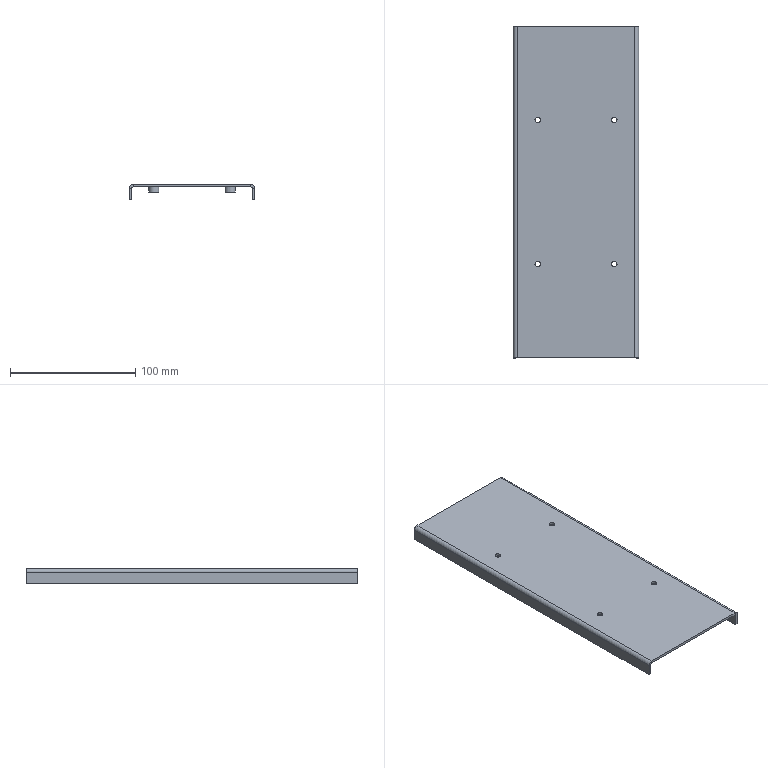Part | SolidWorks | features BaseBody 1 | 1 solid | 54 faces | box 100 x 265 x 12 mm | volume 63166 mm3 | cylinder 28 | plane 26 | commonest cylinder face diameters 4 x8 4.5 x8 8 x8 2 x2 6 x2
STEP:
#1=CARTESIAN_POINT('',(-32.5,-57.5,-6.));
#2=VERTEX_POINT('',#1);
#3=CARTESIAN_POINT('',(-32.5,-57.5,-2.));
#4=VERTEX_POINT('',#3);
#5=CARTESIAN_POINT('',(-32.5,-57.5,-6.));
#6=DIRECTION('',(0.,0.,1.));
#7=VECTOR('',#6,1000.);
#8=LINE('',#5,#7);
#9=EDGE_CURVE('',#2,#4,#8,.T.);
#10=ORIENTED_EDGE('',*,*,#9,.F.);
#11=CARTESIAN_POINT('',(-28.5,-57.5,-6.));
#12=VERTEX_POINT('',#11);
#13=CARTESIAN_POINT('',(-30.5,-57.5,-6.));
#14=DIRECTION('',(0.,0.,-1.));
#15=DIRECTION('',(-1.,0.,0.));
#16=AXIS2_PLACEMENT_3D('',#13,#14,#15);
#17=CIRCLE('',#16,2.);
#18=EDGE_CURVE('',#2,#12,#17,.T.);
#19=ORIENTED_EDGE('',*,*,#18,.T.);
#20=CARTESIAN_POINT('',(-28.5,-57.5,-2.));
#21=VERTEX_POINT('',#20);
#22=CARTESIAN_POINT('',(-28.5,-57.5,-6.));
#23=DIRECTION('',(0.,0.,1.));
#24=VECTOR('',#23,1000.);
#25=LINE('',#22,#24);
#26=EDGE_CURVE('',#12,#21,#25,.T.);
#27=ORIENTED_EDGE('',*,*,#26,.T.);
#28=CARTESIAN_POINT('',(-30.5,-57.5,-2.));
#29=DIRECTION('',(0.,0.,-1.));
#30=DIRECTION('',(-1.,0.,0.));
#31=AXIS2_PLACEMENT_3D('',#28,#29,#30);
#32=CIRCLE('',#31,2.);
#33=EDGE_CURVE('',#4,#21,#32,.T.);
#34=ORIENTED_EDGE('',*,*,#33,.F.);
#35=EDGE_LOOP('',(#10,#19,#27,#34));
#36=FACE_OUTER_BOUND('',#35,.T.);
#37=CARTESIAN_POINT('',(-30.5,-57.5,-6.));
#38=DIRECTION('',(0.,0.,1.));
#39=DIRECTION('',(1.,0.,0.));
#40=AXIS2_PLACEMENT_3D('',#37,#38,#39);
#41=CYLINDRICAL_SURFACE('',#40,2.);
#42=ADVANCED_FACE('',(#36),#41,.F.);
#43=CARTESIAN_POINT('',(-34.5,-57.5,-6.));
#44=VERTEX_POINT('',#43);
#45=CARTESIAN_POINT('',(-34.5,-57.5,-2.));
#46=VERTEX_POINT('',#45);
#47=CARTESIAN_POINT('',(-34.5,-57.5,-6.));
#48=DIRECTION('',(0.,0.,1.));
#49=VECTOR('',#48,1000.);
#50=LINE('',#47,#49);
#51=EDGE_CURVE('',#44,#46,#50,.T.);
#52=ORIENTED_EDGE('',*,*,#51,.F.);
#53=CARTESIAN_POINT('',(-26.5,-57.5,-6.));
#54=VERTEX_POINT('',#53);
#55=CARTESIAN_POINT('',(-30.5,-57.5,-6.));
#56=DIRECTION('',(0.,0.,-1.));
#57=DIRECTION('',(-1.,0.,0.));
#58=AXIS2_PLACEMENT_3D('',#55,#56,#57);
#59=CIRCLE('',#58,4.);
#60=EDGE_CURVE('',#54,#44,#59,.T.);
#61=ORIENTED_EDGE('',*,*,#60,.F.);
#62=CARTESIAN_POINT('',(-26.5,-57.5,-2.));
#63=VERTEX_POINT('',#62);
#64=CARTESIAN_POINT('',(-26.5,-57.5,-6.));
#65=DIRECTION('',(0.,0.,1.));
#66=VECTOR('',#65,1000.);
#67=LINE('',#64,#66);
#68=EDGE_CURVE('',#54,#63,#67,.T.);
#69=ORIENTED_EDGE('',*,*,#68,.T.);
#70=CARTESIAN_POINT('',(-30.5,-57.5,-2.));
#71=DIRECTION('',(0.,0.,-1.));
#72=DIRECTION('',(1.,0.,0.));
#73=AXIS2_PLACEMENT_3D('',#70,#71,#72);
#74=CIRCLE('',#73,4.);
#75=EDGE_CURVE('',#63,#46,#74,.T.);
#76=ORIENTED_EDGE('',*,*,#75,.T.);
#77=EDGE_LOOP('',(#52,#61,#69,#76));
#78=FACE_OUTER_BOUND('',#77,.T.);
#79=CARTESIAN_POINT('',(-30.5,-57.5,-6.));
#80=DIRECTION('',(0.,0.,1.));
#81=DIRECTION('',(1.,0.,0.));
#82=AXIS2_PLACEMENT_3D('',#79,#80,#81);
#83=CYLINDRICAL_SURFACE('',#82,4.);
#84=ADVANCED_FACE('',(#78),#83,.T.);
#85=CARTESIAN_POINT('',(-30.5,-57.5,-6.));
#86=DIRECTION('',(0.,0.,-1.));
#87=DIRECTION('',(-1.,0.,0.));
#88=AXIS2_PLACEMENT_3D('',#85,#86,#87);
#89=CIRCLE('',#88,2.);
#90=EDGE_CURVE('',#12,#2,#89,.T.);
#91=ORIENTED_EDGE('',*,*,#90,.F.);
#92=ORIENTED_EDGE('',*,*,#18,.F.);
#93=EDGE_LOOP('',(#91,#92));
#94=FACE_BOUND('',#93,.T.);
#95=ORIENTED_EDGE('',*,*,#60,.T.);
#96=CARTESIAN_POINT('',(-30.5,-57.5,-6.));
#97=DIRECTION('',(0.,0.,-1.));
#98=DIRECTION('',(-1.,0.,0.));
#99=AXIS2_PLACEMENT_3D('',#96,#97,#98);
#100=CIRCLE('',#99,4.);
#101=EDGE_CURVE('',#44,#54,#100,.T.);
#102=ORIENTED_EDGE('',*,*,#101,.T.);
#103=EDGE_LOOP('',(#95,#102));
#104=FACE_OUTER_BOUND('',#103,.T.);
#105=CARTESIAN_POINT('',(-30.5,-57.5,-6.));
#106=DIRECTION('',(0.,0.,-1.));
#107=DIRECTION('',(0.,-1.,0.));
#108=AXIS2_PLACEMENT_3D('',#105,#106,#107);
#109=PLANE('',#108);
#110=ADVANCED_FACE('',(#94,#104),#109,.T.);
#111=CARTESIAN_POINT('',(-30.5,-57.5,-2.));
#112=DIRECTION('',(0.,0.,-1.));
#113=DIRECTION('',(-1.,0.,0.));
#114=AXIS2_PLACEMENT_3D('',#111,#112,#113);
#115=CIRCLE('',#114,2.);
#116=EDGE_CURVE('',#21,#4,#115,.T.);
#117=ORIENTED_EDGE('',*,*,#116,.T.);
#118=ORIENTED_EDGE('',*,*,#33,.T.);
#119=EDGE_LOOP('',(#117,#118));
#120=FACE_BOUND('',#119,.T.);
#121=CARTESIAN_POINT('',(-28.25,-57.5,-2.));
#122=VERTEX_POINT('',#121);
#123=CARTESIAN_POINT('',(-32.75,-57.5,-2.));
#124=VERTEX_POINT('',#123);
#125=CARTESIAN_POINT('',(-30.5,-57.5,-2.));
#126=DIRECTION('',(0.,0.,1.));
#127=DIRECTION('',(1.,0.,0.));
#128=AXIS2_PLACEMENT_3D('',#125,#126,#127);
#129=CIRCLE('',#128,2.25);
#130=EDGE_CURVE('',#122,#124,#129,.T.);
#131=ORIENTED_EDGE('',*,*,#130,.T.);
#132=CARTESIAN_POINT('',(-30.5,-57.5,-2.));
#133=DIRECTION('',(0.,0.,1.));
#134=DIRECTION('',(1.,0.,0.));
#135=AXIS2_PLACEMENT_3D('',#132,#133,#134);
#136=CIRCLE('',#135,2.25);
#137=EDGE_CURVE('',#124,#122,#136,.T.);
#138=ORIENTED_EDGE('',*,*,#137,.T.);
#139=EDGE_LOOP('',(#131,#138));
#140=FACE_OUTER_BOUND('',#139,.T.);
#141=CARTESIAN_POINT('',(-30.5,-57.5,-2.));
#142=DIRECTION('',(0.,0.,-1.));
#143=DIRECTION('',(0.,-1.,0.));
#144=AXIS2_PLACEMENT_3D('',#141,#142,#143);
#145=PLANE('',#144);
#146=ADVANCED_FACE('',(#120,#140),#145,.F.);
#147=CARTESIAN_POINT('',(28.5,-57.5,-6.));
#148=VERTEX_POINT('',#147);
#149=CARTESIAN_POINT('',(28.5,-57.5,-2.));
#150=VERTEX_POINT('',#149);
#151=CARTESIAN_POINT('',(28.5,-57.5,-6.));
#152=DIRECTION('',(0.,0.,1.));
#153=VECTOR('',#152,1000.);
#154=LINE('',#151,#153);
#155=EDGE_CURVE('',#148,#150,#154,.T.);
#156=ORIENTED_EDGE('',*,*,#155,.F.);
#157=CARTESIAN_POINT('',(32.5,-57.5,-6.));
#158=VERTEX_POINT('',#157);
#159=CARTESIAN_POINT('',(30.5,-57.5,-6.));
#160=DIRECTION('',(0.,0.,-1.));
#161=DIRECTION('',(-1.,0.,0.));
#162=AXIS2_PLACEMENT_3D('',#159,#160,#161);
#163=CIRCLE('',#162,2.);
#164=EDGE_CURVE('',#148,#158,#163,.T.);
#165=ORIENTED_EDGE('',*,*,#164,.T.);
#166=CARTESIAN_POINT('',(32.5,-57.5,-2.));
#167=VERTEX_POINT('',#166);
#168=CARTESIAN_POINT('',(32.5,-57.5,-6.));
#169=DIRECTION('',(0.,0.,1.));
#170=VECTOR('',#169,1000.);
#171=LINE('',#168,#170);
#172=EDGE_CURVE('',#158,#167,#171,.T.);
#173=ORIENTED_EDGE('',*,*,#172,.T.);
#174=CARTESIAN_POINT('',(30.5,-57.5,-2.));
#175=DIRECTION('',(0.,0.,-1.));
#176=DIRECTION('',(-1.,0.,0.));
#177=AXIS2_PLACEMENT_3D('',#174,#175,#176);
#178=CIRCLE('',#177,2.);
#179=EDGE_CURVE('',#150,#167,#178,.T.);
#180=ORIENTED_EDGE('',*,*,#179,.F.);
#181=EDGE_LOOP('',(#156,#165,#173,#180));
#182=FACE_OUTER_BOUND('',#181,.T.);
#183=CARTESIAN_POINT('',(30.5,-57.5,-6.));
#184=DIRECTION('',(0.,0.,1.));
#185=DIRECTION('',(1.,0.,0.));
#186=AXIS2_PLACEMENT_3D('',#183,#184,#185);
#187=CYLINDRICAL_SURFACE('',#186,2.);
#188=ADVANCED_FACE('',(#182),#187,.F.);
#189=CARTESIAN_POINT('',(26.5,-57.5,-6.));
#190=VERTEX_POINT('',#189);
#191=CARTESIAN_POINT('',(26.5,-57.5,-2.));
#192=VERTEX_POINT('',#191);
#193=CARTESIAN_POINT('',(26.5,-57.5,-6.));
#194=DIRECTION('',(0.,0.,1.));
#195=VECTOR('',#194,1000.);
#196=LINE('',#193,#195);
#197=EDGE_CURVE('',#190,#192,#196,.T.);
#198=ORIENTED_EDGE('',*,*,#197,.F.);
#199=CARTESIAN_POINT('',(34.5,-57.5,-6.));
#200=VERTEX_POINT('',#199);
#201=CARTESIAN_POINT('',(30.5,-57.5,-6.));
#202=DIRECTION('',(0.,0.,-1.));
#203=DIRECTION('',(-1.,0.,0.));
#204=AXIS2_PLACEMENT_3D('',#201,#202,#203);
#205=CIRCLE('',#204,4.);
#206=EDGE_CURVE('',#200,#190,#205,.T.);
#207=ORIENTED_EDGE('',*,*,#206,.F.);
#208=CARTESIAN_POINT('',(34.5,-57.5,-2.));
#209=VERTEX_POINT('',#208);
#210=CARTESIAN_POINT('',(34.5,-57.5,-6.));
#211=DIRECTION('',(0.,0.,1.));
#212=VECTOR('',#211,1000.);
#213=LINE('',#210,#212);
#214=EDGE_CURVE('',#200,#209,#213,.T.);
#215=ORIENTED_EDGE('',*,*,#214,.T.);
#216=CARTESIAN_POINT('',(30.5,-57.5,-2.));
#217=DIRECTION('',(0.,0.,-1.));
#218=DIRECTION('',(1.,0.,0.));
#219=AXIS2_PLACEMENT_3D('',#216,#217,#218);
#220=CIRCLE('',#219,4.);
#221=EDGE_CURVE('',#209,#192,#220,.T.);
#222=ORIENTED_EDGE('',*,*,#221,.T.);
#223=EDGE_LOOP('',(#198,#207,#215,#222));
#224=FACE_OUTER_BOUND('',#223,.T.);
#225=CARTESIAN_POINT('',(30.5,-57.5,-6.));
#226=DIRECTION('',(0.,0.,1.));
#227=DIRECTION('',(1.,0.,0.));
#228=AXIS2_PLACEMENT_3D('',#225,#226,#227);
#229=CYLINDRICAL_SURFACE('',#228,4.);
#230=ADVANCED_FACE('',(#224),#229,.T.);
#231=CARTESIAN_POINT('',(30.5,-57.5,-6.));
#232=DIRECTION('',(0.,0.,-1.));
#233=DIRECTION('',(-1.,0.,0.));
#234=AXIS2_PLACEMENT_3D('',#231,#232,#233);
#235=CIRCLE('',#234,2.);
#236=EDGE_CURVE('',#158,#148,#235,.T.);
#237=ORIENTED_EDGE('',*,*,#236,.F.);
#238=ORIENTED_EDGE('',*,*,#164,.F.);
#239=EDGE_LOOP('',(#237,#238));
#240=FACE_BOUND('',#239,.T.);
#241=ORIENTED_EDGE('',*,*,#206,.T.);
#242=CARTESIAN_POINT('',(30.5,-57.5,-6.));
#243=DIRECTION('',(0.,0.,-1.));
#244=DIRECTION('',(-1.,0.,0.));
#245=AXIS2_PLACEMENT_3D('',#242,#243,#244);
#246=CIRCLE('',#245,4.);
#247=EDGE_CURVE('',#190,#200,#246,.T.);
#248=ORIENTED_EDGE('',*,*,#247,.T.);
#249=EDGE_LOOP('',(#241,#248));
#250=FACE_OUTER_BOUND('',#249,.T.);
#251=CARTESIAN_POINT('',(30.5,-57.5,-6.));
#252=DIRECTION('',(0.,0.,-1.));
#253=DIRECTION('',(0.,-1.,0.));
#254=AXIS2_PLACEMENT_3D('',#251,#252,#253);
#255=PLANE('',#254);
#256=ADVANCED_FACE('',(#240,#250),#255,.T.);
#257=CARTESIAN_POINT('',(30.5,-57.5,-2.));
#258=DIRECTION('',(0.,0.,-1.));
#259=DIRECTION('',(-1.,0.,0.));
#260=AXIS2_PLACEMENT_3D('',#257,#258,#259);
#261=CIRCLE('',#260,2.);
#262=EDGE_CURVE('',#167,#150,#261,.T.);
#263=ORIENTED_EDGE('',*,*,#262,.T.);
#264=ORIENTED_EDGE('',*,*,#179,.T.);
#265=EDGE_LOOP('',(#263,#264));
#266=FACE_BOUND('',#265,.T.);
#267=CARTESIAN_POINT('',(32.75,-57.5,-2.));
#268=VERTEX_POINT('',#267);
#269=CARTESIAN_POINT('',(28.25,-57.5,-2.));
#270=VERTEX_POINT('',#269);
#271=CARTESIAN_POINT('',(30.5,-57.5,-2.));
#272=DIRECTION('',(0.,0.,1.));
#273=DIRECTION('',(1.,0.,0.));
#274=AXIS2_PLACEMENT_3D('',#271,#272,#273);
#275=CIRCLE('',#274,2.25);
#276=EDGE_CURVE('',#268,#270,#275,.T.);
#277=ORIENTED_EDGE('',*,*,#276,.T.);
#278=CARTESIAN_POINT('',(30.5,-57.5,-2.));
#279=DIRECTION('',(0.,0.,1.));
#280=DIRECTION('',(1.,0.,0.));
#281=AXIS2_PLACEMENT_3D('',#278,#279,#280);
#282=CIRCLE('',#281,2.25);
#283=EDGE_CURVE('',#270,#268,#282,.T.);
#284=ORIENTED_EDGE('',*,*,#283,.T.);
#285=EDGE_LOOP('',(#277,#284));
#286=FACE_OUTER_BOUND('',#285,.T.);
#287=CARTESIAN_POINT('',(30.5,-57.5,-2.));
#288=DIRECTION('',(0.,0.,-1.));
#289=DIRECTION('',(0.,-1.,0.));
#290=AXIS2_PLACEMENT_3D('',#287,#288,#289);
#291=PLANE('',#290);
#292=ADVANCED_FACE('',(#266,#286),#291,.F.);
#293=CARTESIAN_POINT('',(-32.5,57.5,-6.));
#294=VERTEX_POINT('',#293);
#295=CARTESIAN_POINT('',(-32.5,57.5,-2.));
#296=VERTEX_POINT('',#295);
#297=CARTESIAN_POINT('',(-32.5,57.5,-6.));
#298=DIRECTION('',(0.,0.,1.));
#299=VECTOR('',#298,1000.);
#300=LINE('',#297,#299);
#301=EDGE_CURVE('',#294,#296,#300,.T.);
#302=ORIENTED_EDGE('',*,*,#301,.F.);
#303=CARTESIAN_POINT('',(-28.5,57.5,-6.));
#304=VERTEX_POINT('',#303);
#305=CARTESIAN_POINT('',(-30.5,57.5,-6.));
#306=DIRECTION('',(0.,0.,-1.));
#307=DIRECTION('',(-1.,0.,0.));
#308=AXIS2_PLACEMENT_3D('',#305,#306,#307);
#309=CIRCLE('',#308,2.);
#310=EDGE_CURVE('',#294,#304,#309,.T.);
#311=ORIENTED_EDGE('',*,*,#310,.T.);
#312=CARTESIAN_POINT('',(-28.5,57.5,-2.));
#313=VERTEX_POINT('',#312);
#314=CARTESIAN_POINT('',(-28.5,57.5,-6.));
#315=DIRECTION('',(0.,0.,1.));
#316=VECTOR('',#315,1000.);
#317=LINE('',#314,#316);
#318=EDGE_CURVE('',#304,#313,#317,.T.);
#319=ORIENTED_EDGE('',*,*,#318,.T.);
#320=CARTESIAN_POINT('',(-30.5,57.5,-2.));
#321=DIRECTION('',(0.,0.,-1.));
#322=DIRECTION('',(-1.,0.,0.));
#323=AXIS2_PLACEMENT_3D('',#320,#321,#322);
#324=CIRCLE('',#323,2.);
#325=EDGE_CURVE('',#296,#313,#324,.T.);
#326=ORIENTED_EDGE('',*,*,#325,.F.);
#327=EDGE_LOOP('',(#302,#311,#319,#326));
#328=FACE_OUTER_BOUND('',#327,.T.);
#329=CARTESIAN_POINT('',(-30.5,57.5,-6.));
#330=DIRECTION('',(0.,0.,1.));
#331=DIRECTION('',(1.,0.,0.));
#332=AXIS2_PLACEMENT_3D('',#329,#330,#331);
#333=CYLINDRICAL_SURFACE('',#332,2.);
#334=ADVANCED_FACE('',(#328),#333,.F.);
#335=CARTESIAN_POINT('',(-34.5,57.5,-6.));
#336=VERTEX_POINT('',#335);
#337=CARTESIAN_POINT('',(-34.5,57.5,-2.));
#338=VERTEX_POINT('',#337);
#339=CARTESIAN_POINT('',(-34.5,57.5,-6.));
#340=DIRECTION('',(0.,0.,1.));
#341=VECTOR('',#340,1000.);
#342=LINE('',#339,#341);
#343=EDGE_CURVE('',#336,#338,#342,.T.);
#344=ORIENTED_EDGE('',*,*,#343,.F.);
#345=CARTESIAN_POINT('',(-26.5,57.5,-6.));
#346=VERTEX_POINT('',#345);
#347=CARTESIAN_POINT('',(-30.5,57.5,-6.));
#348=DIRECTION('',(0.,0.,-1.));
#349=DIRECTION('',(-1.,0.,0.));
#350=AXIS2_PLACEMENT_3D('',#347,#348,#349);
#351=CIRCLE('',#350,4.);
#352=EDGE_CURVE('',#346,#336,#351,.T.);
#353=ORIENTED_EDGE('',*,*,#352,.F.);
#354=CARTESIAN_POINT('',(-26.5,57.5,-2.));
#355=VERTEX_POINT('',#354);
#356=CARTESIAN_POINT('',(-26.5,57.5,-6.));
#357=DIRECTION('',(0.,0.,1.));
#358=VECTOR('',#357,1000.);
#359=LINE('',#356,#358);
#360=EDGE_CURVE('',#346,#355,#359,.T.);
#361=ORIENTED_EDGE('',*,*,#360,.T.);
#362=CARTESIAN_POINT('',(-30.5,57.5,-2.));
#363=DIRECTION('',(0.,0.,-1.));
#364=DIRECTION('',(1.,0.,0.));
#365=AXIS2_PLACEMENT_3D('',#362,#363,#364);
#366=CIRCLE('',#365,4.);
#367=EDGE_CURVE('',#355,#338,#366,.T.);
#368=ORIENTED_EDGE('',*,*,#367,.T.);
#369=EDGE_LOOP('',(#344,#353,#361,#368));
#370=FACE_OUTER_BOUND('',#369,.T.);
#371=CARTESIAN_POINT('',(-30.5,57.5,-6.));
#372=DIRECTION('',(0.,0.,1.));
#373=DIRECTION('',(1.,0.,0.));
#374=AXIS2_PLACEMENT_3D('',#371,#372,#373);
#375=CYLINDRICAL_SURFACE('',#374,4.);
#376=ADVANCED_FACE('',(#370),#375,.T.);
#377=CARTESIAN_POINT('',(-30.5,57.5,-6.));
#378=DIRECTION('',(0.,0.,-1.));
#379=DIRECTION('',(-1.,0.,0.));
#380=AXIS2_PLACEMENT_3D('',#377,#378,#379);
#381=CIRCLE('',#380,2.);
#382=EDGE_CURVE('',#304,#294,#381,.T.);
#383=ORIENTED_EDGE('',*,*,#382,.F.);
#384=ORIENTED_EDGE('',*,*,#310,.F.);
#385=EDGE_LOOP('',(#383,#384));
#386=FACE_BOUND('',#385,.T.);
#387=ORIENTED_EDGE('',*,*,#352,.T.);
#388=CARTESIAN_POINT('',(-30.5,57.5,-6.));
#389=DIRECTION('',(0.,0.,-1.));
#390=DIRECTION('',(-1.,0.,0.));
#391=AXIS2_PLACEMENT_3D('',#388,#389,#390);
#392=CIRCLE('',#391,4.);
#393=EDGE_CURVE('',#336,#346,#392,.T.);
#394=ORIENTED_EDGE('',*,*,#393,.T.);
#395=EDGE_LOOP('',(#387,#394));
#396=FACE_OUTER_BOUND('',#395,.T.);
#397=CARTESIAN_POINT('',(-30.5,57.5,-6.));
#398=DIRECTION('',(0.,0.,-1.));
#399=DIRECTION('',(0.,-1.,0.));
#400=AXIS2_PLACEMENT_3D('',#397,#398,#399);
#401=PLANE('',#400);
#402=ADVANCED_FACE('',(#386,#396),#401,.T.);
#403=CARTESIAN_POINT('',(-30.5,57.5,-2.));
#404=DIRECTION('',(0.,0.,-1.));
#405=DIRECTION('',(-1.,0.,0.));
#406=AXIS2_PLACEMENT_3D('',#403,#404,#405);
#407=CIRCLE('',#406,2.);
#408=EDGE_CURVE('',#313,#296,#407,.T.);
#409=ORIENTED_EDGE('',*,*,#408,.T.);
#410=ORIENTED_EDGE('',*,*,#325,.T.);
#411=EDGE_LOOP('',(#409,#410));
#412=FACE_BOUND('',#411,.T.);
#413=CARTESIAN_POINT('',(-28.25,57.5,-2.));
#414=VERTEX_POINT('',#413);
#415=CARTESIAN_POINT('',(-32.75,57.5,-2.));
#416=VERTEX_POINT('',#415);
#417=CARTESIAN_POINT('',(-30.5,57.5,-2.));
#418=DIRECTION('',(0.,0.,1.));
#419=DIRECTION('',(1.,0.,0.));
#420=AXIS2_PLACEMENT_3D('',#417,#418,#419);
#421=CIRCLE('',#420,2.25);
#422=EDGE_CURVE('',#414,#416,#421,.T.);
#423=ORIENTED_EDGE('',*,*,#422,.T.);
#424=CARTESIAN_POINT('',(-30.5,57.5,-2.));
#425=DIRECTION('',(0.,0.,1.));
#426=DIRECTION('',(1.,0.,0.));
#427=AXIS2_PLACEMENT_3D('',#424,#425,#426);
#428=CIRCLE('',#427,2.25);
#429=EDGE_CURVE('',#416,#414,#428,.T.);
#430=ORIENTED_EDGE('',*,*,#429,.T.);
#431=EDGE_LOOP('',(#423,#430));
#432=FACE_OUTER_BOUND('',#431,.T.);
#433=CARTESIAN_POINT('',(-30.5,57.5,-2.));
#434=DIRECTION('',(0.,0.,-1.));
#435=DIRECTION('',(0.,-1.,0.));
#436=AXIS2_PLACEMENT_3D('',#433,#434,#435);
#437=PLANE('',#436);
#438=ADVANCED_FACE('',(#412,#432),#437,.F.);
#439=CARTESIAN_POINT('',(28.5,57.5,-6.));
#440=VERTEX_POINT('',#439);
#441=CARTESIAN_POINT('',(28.5,57.5,-2.));
#442=VERTEX_POINT('',#441);
#443=CARTESIAN_POINT('',(28.5,57.5,-6.));
#444=DIRECTION('',(0.,0.,1.));
#445=VECTOR('',#444,1000.);
#446=LINE('',#443,#445);
#447=EDGE_CURVE('',#440,#442,#446,.T.);
#448=ORIENTED_EDGE('',*,*,#447,.F.);
#449=CARTESIAN_POINT('',(32.5,57.5,-6.));
#450=VERTEX_POINT('',#449);
#451=CARTESIAN_POINT('',(30.5,57.5,-6.));
#452=DIRECTION('',(0.,0.,-1.));
#453=DIRECTION('',(-1.,0.,0.));
#454=AXIS2_PLACEMENT_3D('',#451,#452,#453);
#455=CIRCLE('',#454,2.);
#456=EDGE_CURVE('',#440,#450,#455,.T.);
#457=ORIENTED_EDGE('',*,*,#456,.T.);
#458=CARTESIAN_POINT('',(32.5,57.5,-2.));
#459=VERTEX_POINT('',#458);
#460=CARTESIAN_POINT('',(32.5,57.5,-6.));
#461=DIRECTION('',(0.,0.,1.));
#462=VECTOR('',#461,1000.);
#463=LINE('',#460,#462);
#464=EDGE_CURVE('',#450,#459,#463,.T.);
#465=ORIENTED_EDGE('',*,*,#464,.T.);
#466=CARTESIAN_POINT('',(30.5,57.5,-2.));
#467=DIRECTION('',(0.,0.,-1.));
#468=DIRECTION('',(-1.,0.,0.));
#469=AXIS2_PLACEMENT_3D('',#466,#467,#468);
#470=CIRCLE('',#469,2.);
#471=EDGE_CURVE('',#442,#459,#470,.T.);
#472=ORIENTED_EDGE('',*,*,#471,.F.);
#473=EDGE_LOOP('',(#448,#457,#465,#472));
#474=FACE_OUTER_BOUND('',#473,.T.);
#475=CARTESIAN_POINT('',(30.5,57.5,-6.));
#476=DIRECTION('',(0.,0.,1.));
#477=DIRECTION('',(1.,0.,0.));
#478=AXIS2_PLACEMENT_3D('',#475,#476,#477);
#479=CYLINDRICAL_SURFACE('',#478,2.);
#480=ADVANCED_FACE('',(#474),#479,.F.);
#481=CARTESIAN_POINT('',(26.5,57.5,-6.));
#482=VERTEX_POINT('',#481);
#483=CARTESIAN_POINT('',(26.5,57.5,-2.));
#484=VERTEX_POINT('',#483);
#485=CARTESIAN_POINT('',(26.5,57.5,-6.));
#486=DIRECTION('',(0.,0.,1.));
#487=VECTOR('',#486,1000.);
#488=LINE('',#485,#487);
#489=EDGE_CURVE('',#482,#484,#488,.T.);
#490=ORIENTED_EDGE('',*,*,#489,.F.);
#491=CARTESIAN_POINT('',(34.5,57.5,-6.));
#492=VERTEX_POINT('',#491);
#493=CARTESIAN_POINT('',(30.5,57.5,-6.));
#494=DIRECTION('',(0.,0.,-1.));
#495=DIRECTION('',(-1.,0.,0.));
#496=AXIS2_PLACEMENT_3D('',#493,#494,#495);
#497=CIRCLE('',#496,4.);
#498=EDGE_CURVE('',#492,#482,#497,.T.);
#499=ORIENTED_EDGE('',*,*,#498,.F.);
#500=CARTESIAN_POINT('',(34.5,57.5,-2.));
#501=VERTEX_POINT('',#500);
#502=CARTESIAN_POINT('',(34.5,57.5,-6.));
#503=DIRECTION('',(0.,0.,1.));
#504=VECTOR('',#503,1000.);
#505=LINE('',#502,#504);
#506=EDGE_CURVE('',#492,#501,#505,.T.);
#507=ORIENTED_EDGE('',*,*,#506,.T.);
#508=CARTESIAN_POINT('',(30.5,57.5,-2.));
#509=DIRECTION('',(0.,0.,-1.));
#510=DIRECTION('',(1.,0.,0.));
#511=AXIS2_PLACEMENT_3D('',#508,#509,#510);
#512=CIRCLE('',#511,4.);
#513=EDGE_CURVE('',#501,#484,#512,.T.);
#514=ORIENTED_EDGE('',*,*,#513,.T.);
#515=EDGE_LOOP('',(#490,#499,#507,#514));
#516=FACE_OUTER_BOUND('',#515,.T.);
#517=CARTESIAN_POINT('',(30.5,57.5,-6.));
#518=DIRECTION('',(0.,0.,1.));
#519=DIRECTION('',(1.,0.,0.));
#520=AXIS2_PLACEMENT_3D('',#517,#518,#519);
#521=CYLINDRICAL_SURFACE('',#520,4.);
#522=ADVANCED_FACE('',(#516),#521,.T.);
#523=CARTESIAN_POINT('',(30.5,57.5,-6.));
#524=DIRECTION('',(0.,0.,-1.));
#525=DIRECTION('',(-1.,0.,0.));
#526=AXIS2_PLACEMENT_3D('',#523,#524,#525);
#527=CIRCLE('',#526,2.);
#528=EDGE_CURVE('',#450,#440,#527,.T.);
#529=ORIENTED_EDGE('',*,*,#528,.F.);
#530=ORIENTED_EDGE('',*,*,#456,.F.);
#531=EDGE_LOOP('',(#529,#530));
#532=FACE_BOUND('',#531,.T.);
#533=ORIENTED_EDGE('',*,*,#498,.T.);
#534=CARTESIAN_POINT('',(30.5,57.5,-6.));
#535=DIRECTION('',(0.,0.,-1.));
#536=DIRECTION('',(-1.,0.,0.));
#537=AXIS2_PLACEMENT_3D('',#534,#535,#536);
#538=CIRCLE('',#537,4.);
#539=EDGE_CURVE('',#482,#492,#538,.T.);
#540=ORIENTED_EDGE('',*,*,#539,.T.);
#541=EDGE_LOOP('',(#533,#540));
#542=FACE_OUTER_BOUND('',#541,.T.);
#543=CARTESIAN_POINT('',(30.5,57.5,-6.));
#544=DIRECTION('',(0.,0.,-1.));
#545=DIRECTION('',(0.,-1.,0.));
#546=AXIS2_PLACEMENT_3D('',#543,#544,#545);
#547=PLANE('',#546);
#548=ADVANCED_FACE('',(#532,#542),#547,.T.);
#549=CARTESIAN_POINT('',(30.5,57.5,-2.));
#550=DIRECTION('',(0.,0.,-1.));
#551=DIRECTION('',(-1.,0.,0.));
#552=AXIS2_PLACEMENT_3D('',#549,#550,#551);
#553=CIRCLE('',#552,2.);
#554=EDGE_CURVE('',#459,#442,#553,.T.);
#555=ORIENTED_EDGE('',*,*,#554,.T.);
#556=ORIENTED_EDGE('',*,*,#471,.T.);
#557=EDGE_LOOP('',(#555,#556));
#558=FACE_BOUND('',#557,.T.);
#559=CARTESIAN_POINT('',(32.75,57.5,-2.));
#560=VERTEX_POINT('',#559);
#561=CARTESIAN_POINT('',(28.25,57.5,-2.));
#562=VERTEX_POINT('',#561);
#563=CARTESIAN_POINT('',(30.5,57.5,-2.));
#564=DIRECTION('',(0.,0.,1.));
#565=DIRECTION('',(1.,0.,0.));
#566=AXIS2_PLACEMENT_3D('',#563,#564,#565);
#567=CIRCLE('',#566,2.25);
#568=EDGE_CURVE('',#560,#562,#567,.T.);
#569=ORIENTED_EDGE('',*,*,#568,.T.);
#570=CARTESIAN_POINT('',(30.5,57.5,-2.));
#571=DIRECTION('',(0.,0.,1.));
#572=DIRECTION('',(1.,0.,0.));
#573=AXIS2_PLACEMENT_3D('',#570,#571,#572);
#574=CIRCLE('',#573,2.25);
#575=EDGE_CURVE('',#562,#560,#574,.T.);
#576=ORIENTED_EDGE('',*,*,#575,.T.);
#577=EDGE_LOOP('',(#569,#576));
#578=FACE_OUTER_BOUND('',#577,.T.);
#579=CARTESIAN_POINT('',(30.5,57.5,-2.));
#580=DIRECTION('',(0.,0.,-1.));
#581=DIRECTION('',(0.,-1.,0.));
#582=AXIS2_PLACEMENT_3D('',#579,#580,#581);
#583=PLANE('',#582);
#584=ADVANCED_FACE('',(#558,#578),#583,.F.);
#585=CARTESIAN_POINT('',(-32.75,57.5,0.));
#586=VERTEX_POINT('',#585);
#587=CARTESIAN_POINT('',(-32.75,57.5,-2.));
#588=DIRECTION('',(0.,0.,1.));
#589=VECTOR('',#588,1000.);
#590=LINE('',#587,#589);
#591=EDGE_CURVE('',#416,#586,#590,.T.);
#592=ORIENTED_EDGE('',*,*,#591,.F.);
#593=ORIENTED_EDGE('',*,*,#422,.F.);
#594=CARTESIAN_POINT('',(-28.25,57.5,0.));
#595=VERTEX_POINT('',#594);
#596=CARTESIAN_POINT('',(-28.25,57.5,-2.));
#597=DIRECTION('',(0.,0.,1.));
#598=VECTOR('',#597,1000.);
#599=LINE('',#596,#598);
#600=EDGE_CURVE('',#414,#595,#599,.T.);
#601=ORIENTED_EDGE('',*,*,#600,.T.);
#602=CARTESIAN_POINT('',(-30.5,57.5,0.));
#603=DIRECTION('',(0.,0.,1.));
#604=DIRECTION('',(1.,0.,0.));
#605=AXIS2_PLACEMENT_3D('',#602,#603,#604);
#606=CIRCLE('',#605,2.25);
#607=EDGE_CURVE('',#595,#586,#606,.T.);
#608=ORIENTED_EDGE('',*,*,#607,.T.);
#609=EDGE_LOOP('',(#592,#593,#601,#608));
#610=FACE_OUTER_BOUND('',#609,.T.);
#611=CARTESIAN_POINT('',(-30.5,57.5,-2.));
#612=DIRECTION('',(0.,0.,1.));
#613=DIRECTION('',(1.,0.,0.));
#614=AXIS2_PLACEMENT_3D('',#611,#612,#613);
#615=CYLINDRICAL_SURFACE('',#614,2.25);
#616=ADVANCED_FACE('',(#610),#615,.F.);
#617=CARTESIAN_POINT('',(28.25,-57.5,0.));
#618=VERTEX_POINT('',#617);
#619=CARTESIAN_POINT('',(28.25,-57.5,-2.));
#620=DIRECTION('',(0.,0.,1.));
#621=VECTOR('',#620,1000.);
#622=LINE('',#619,#621);
#623=EDGE_CURVE('',#270,#618,#622,.T.);
#624=ORIENTED_EDGE('',*,*,#623,.F.);
#625=ORIENTED_EDGE('',*,*,#276,.F.);
#626=CARTESIAN_POINT('',(32.75,-57.5,0.));
#627=VERTEX_POINT('',#626);
#628=CARTESIAN_POINT('',(32.75,-57.5,-2.));
#629=DIRECTION('',(0.,0.,1.));
#630=VECTOR('',#629,1000.);
#631=LINE('',#628,#630);
#632=EDGE_CURVE('',#268,#627,#631,.T.);
#633=ORIENTED_EDGE('',*,*,#632,.T.);
#634=CARTESIAN_POINT('',(30.5,-57.5,0.));
#635=DIRECTION('',(0.,0.,1.));
#636=DIRECTION('',(1.,0.,0.));
#637=AXIS2_PLACEMENT_3D('',#634,#635,#636);
#638=CIRCLE('',#637,2.25);
#639=EDGE_CURVE('',#627,#618,#638,.T.);
#640=ORIENTED_EDGE('',*,*,#639,.T.);
#641=EDGE_LOOP('',(#624,#625,#633,#640));
#642=FACE_OUTER_BOUND('',#641,.T.);
#643=CARTESIAN_POINT('',(30.5,-57.5,-2.));
#644=DIRECTION('',(0.,0.,1.));
#645=DIRECTION('',(1.,0.,0.));
#646=AXIS2_PLACEMENT_3D('',#643,#644,#645);
#647=CYLINDRICAL_SURFACE('',#646,2.25);
#648=ADVANCED_FACE('',(#642),#647,.F.);
#649=CARTESIAN_POINT('',(-32.75,-57.5,0.));
#650=VERTEX_POINT('',#649);
#651=CARTESIAN_POINT('',(-32.75,-57.5,-2.));
#652=DIRECTION('',(0.,0.,1.));
#653=VECTOR('',#652,1000.);
#654=LINE('',#651,#653);
#655=EDGE_CURVE('',#124,#650,#654,.T.);
#656=ORIENTED_EDGE('',*,*,#655,.F.);
#657=ORIENTED_EDGE('',*,*,#130,.F.);
#658=CARTESIAN_POINT('',(-28.25,-57.5,0.));
#659=VERTEX_POINT('',#658);
#660=CARTESIAN_POINT('',(-28.25,-57.5,-2.));
#661=DIRECTION('',(0.,0.,1.));
#662=VECTOR('',#661,1000.);
#663=LINE('',#660,#662);
#664=EDGE_CURVE('',#122,#659,#663,.T.);
#665=ORIENTED_EDGE('',*,*,#664,.T.);
#666=CARTESIAN_POINT('',(-30.5,-57.5,0.));
#667=DIRECTION('',(0.,0.,1.));
#668=DIRECTION('',(1.,0.,0.));
#669=AXIS2_PLACEMENT_3D('',#666,#667,#668);
#670=CIRCLE('',#669,2.25);
#671=EDGE_CURVE('',#659,#650,#670,.T.);
#672=ORIENTED_EDGE('',*,*,#671,.T.);
#673=EDGE_LOOP('',(#656,#657,#665,#672));
#674=FACE_OUTER_BOUND('',#673,.T.);
#675=CARTESIAN_POINT('',(-30.5,-57.5,-2.));
#676=DIRECTION('',(0.,0.,1.));
#677=DIRECTION('',(1.,0.,0.));
#678=AXIS2_PLACEMENT_3D('',#675,#676,#677);
#679=CYLINDRICAL_SURFACE('',#678,2.25);
#680=ADVANCED_FACE('',(#674),#679,.F.);
#681=CARTESIAN_POINT('',(28.25,57.5,0.));
#682=VERTEX_POINT('',#681);
#683=CARTESIAN_POINT('',(28.25,57.5,-2.));
#684=DIRECTION('',(0.,0.,1.));
#685=VECTOR('',#684,1000.);
#686=LINE('',#683,#685);
#687=EDGE_CURVE('',#562,#682,#686,.T.);
#688=ORIENTED_EDGE('',*,*,#687,.F.);
#689=ORIENTED_EDGE('',*,*,#568,.F.);
#690=CARTESIAN_POINT('',(32.75,57.5,0.));
#691=VERTEX_POINT('',#690);
#692=CARTESIAN_POINT('',(32.75,57.5,-2.));
#693=DIRECTION('',(0.,0.,1.));
#694=VECTOR('',#693,1000.);
#695=LINE('',#692,#694);
#696=EDGE_CURVE('',#560,#691,#695,.T.);
#697=ORIENTED_EDGE('',*,*,#696,.T.);
#698=CARTESIAN_POINT('',(30.5,57.5,0.));
#699=DIRECTION('',(0.,0.,1.));
#700=DIRECTION('',(1.,0.,0.));
#701=AXIS2_PLACEMENT_3D('',#698,#699,#700);
#702=CIRCLE('',#701,2.25);
#703=EDGE_CURVE('',#691,#682,#702,.T.);
#704=ORIENTED_EDGE('',*,*,#703,.T.);
#705=EDGE_LOOP('',(#688,#689,#697,#704));
#706=FACE_OUTER_BOUND('',#705,.T.);
#707=CARTESIAN_POINT('',(30.5,57.5,-2.));
#708=DIRECTION('',(0.,0.,1.));
#709=DIRECTION('',(1.,0.,0.));
#710=AXIS2_PLACEMENT_3D('',#707,#708,#709);
#711=CYLINDRICAL_SURFACE('',#710,2.25);
#712=ADVANCED_FACE('',(#706),#711,.F.);
#713=CARTESIAN_POINT('',(-48.,-132.5,-12.));
#714=VERTEX_POINT('',#713);
#715=CARTESIAN_POINT('',(-48.,132.5,-12.));
#716=VERTEX_POINT('',#715);
#717=CARTESIAN_POINT('',(-48.,0.,-12.));
#718=DIRECTION('',(0.,1.,0.));
#719=VECTOR('',#718,1000.);
#720=LINE('',#717,#719);
#721=EDGE_CURVE('',#714,#716,#720,.T.);
#722=ORIENTED_EDGE('',*,*,#721,.F.);
#723=CARTESIAN_POINT('',(-50.,-132.5,-12.));
#724=VERTEX_POINT('',#723);
#725=CARTESIAN_POINT('',(-50.,-132.5,-12.));
#726=DIRECTION('',(1.,0.,0.));
#727=VECTOR('',#726,1000.);
#728=LINE('',#725,#727);
#729=EDGE_CURVE('',#724,#714,#728,.T.);
#730=ORIENTED_EDGE('',*,*,#729,.F.);
#731=CARTESIAN_POINT('',(-50.,132.5,-12.));
#732=VERTEX_POINT('',#731);
#733=CARTESIAN_POINT('',(-50.,-132.5,-12.));
#734=DIRECTION('',(0.,1.,0.));
#735=VECTOR('',#734,1000.);
#736=LINE('',#733,#735);
#737=EDGE_CURVE('',#724,#732,#736,.T.);
#738=ORIENTED_EDGE('',*,*,#737,.T.);
#739=CARTESIAN_POINT('',(-50.,132.5,-12.));
#740=DIRECTION('',(1.,0.,0.));
#741=VECTOR('',#740,1000.);
#742=LINE('',#739,#741);
#743=EDGE_CURVE('',#732,#716,#742,.T.);
#744=ORIENTED_EDGE('',*,*,#743,.T.);
#745=EDGE_LOOP('',(#722,#730,#738,#744));
#746=FACE_OUTER_BOUND('',#745,.T.);
#747=CARTESIAN_POINT('',(-50.,-132.5,-12.));
#748=DIRECTION('',(0.,0.,-1.));
#749=DIRECTION('',(-1.,0.,0.));
#750=AXIS2_PLACEMENT_3D('',#747,#748,#749);
#751=PLANE('',#750);
#752=ADVANCED_FACE('',(#746),#751,.T.);
#753=CARTESIAN_POINT('',(-48.,132.5,-3.));
#754=VERTEX_POINT('',#753);
#755=CARTESIAN_POINT('',(-48.,132.5,0.));
#756=DIRECTION('',(0.,0.,1.));
#757=VECTOR('',#756,1000.);
#758=LINE('',#755,#757);
#759=EDGE_CURVE('',#716,#754,#758,.T.);
#760=ORIENTED_EDGE('',*,*,#759,.T.);
#761=CARTESIAN_POINT('',(-48.,-132.5,-3.));
#762=VERTEX_POINT('',#761);
#763=CARTESIAN_POINT('',(-48.,-132.5,-3.));
#764=DIRECTION('',(0.,1.,0.));
#765=VECTOR('',#764,1000.);
#766=LINE('',#763,#765);
#767=EDGE_CURVE('',#762,#754,#766,.T.);
#768=ORIENTED_EDGE('',*,*,#767,.F.);
#769=CARTESIAN_POINT('',(-48.,-132.5,0.));
#770=DIRECTION('',(0.,0.,-1.));
#771=VECTOR('',#770,1000.);
#772=LINE('',#769,#771);
#773=EDGE_CURVE('',#762,#714,#772,.T.);
#774=ORIENTED_EDGE('',*,*,#773,.T.);
#775=ORIENTED_EDGE('',*,*,#721,.T.);
#776=EDGE_LOOP('',(#760,#768,#774,#775));
#777=FACE_OUTER_BOUND('',#776,.T.);
#778=CARTESIAN_POINT('',(-48.,0.,0.));
#779=DIRECTION('',(1.,0.,0.));
#780=DIRECTION('',(0.,0.,-1.));
#781=AXIS2_PLACEMENT_3D('',#778,#779,#780);
#782=PLANE('',#781);
#783=ADVANCED_FACE('',(#777),#782,.T.);
#784=CARTESIAN_POINT('',(-50.,132.5,-3.));
#785=VERTEX_POINT('',#784);
#786=CARTESIAN_POINT('',(-50.,-132.5,-3.));
#787=VERTEX_POINT('',#786);
#788=CARTESIAN_POINT('',(-50.,-132.5,-3.));
#789=DIRECTION('',(0.,-1.,0.));
#790=VECTOR('',#789,1000.);
#791=LINE('',#788,#790);
#792=EDGE_CURVE('',#785,#787,#791,.T.);
#793=ORIENTED_EDGE('',*,*,#792,.F.);
#794=CARTESIAN_POINT('',(-50.,132.5,-12.));
#795=DIRECTION('',(0.,0.,1.));
#796=VECTOR('',#795,1000.);
#797=LINE('',#794,#796);
#798=EDGE_CURVE('',#732,#785,#797,.T.);
#799=ORIENTED_EDGE('',*,*,#798,.F.);
#800=ORIENTED_EDGE('',*,*,#737,.F.);
#801=CARTESIAN_POINT('',(-50.,-132.5,-2.));
#802=DIRECTION('',(0.,0.,-1.));
#803=VECTOR('',#802,1000.);
#804=LINE('',#801,#803);
#805=EDGE_CURVE('',#787,#724,#804,.T.);
#806=ORIENTED_EDGE('',*,*,#805,.F.);
#807=EDGE_LOOP('',(#793,#799,#800,#806));
#808=FACE_OUTER_BOUND('',#807,.T.);
#809=CARTESIAN_POINT('',(-50.,0.,0.));
#810=DIRECTION('',(1.,0.,0.));
#811=DIRECTION('',(0.,0.,-1.));
#812=AXIS2_PLACEMENT_3D('',#809,#810,#811);
#813=PLANE('',#812);
#814=ADVANCED_FACE('',(#808),#813,.F.);
#815=ORIENTED_EDGE('',*,*,#798,.T.);
#816=CARTESIAN_POINT('',(-48.,132.5,-3.));
#817=DIRECTION('',(-1.,0.,0.));
#818=VECTOR('',#817,1000.);
#819=LINE('',#816,#818);
#820=EDGE_CURVE('',#754,#785,#819,.T.);
#821=ORIENTED_EDGE('',*,*,#820,.F.);
#822=ORIENTED_EDGE('',*,*,#759,.F.);
#823=ORIENTED_EDGE('',*,*,#743,.F.);
#824=EDGE_LOOP('',(#815,#821,#822,#823));
#825=FACE_OUTER_BOUND('',#824,.T.);
#826=CARTESIAN_POINT('',(-50.,132.5,-12.));
#827=DIRECTION('',(0.,1.,0.));
#828=DIRECTION('',(1.,0.,0.));
#829=AXIS2_PLACEMENT_3D('',#826,#827,#828);
#830=PLANE('',#829);
#831=ADVANCED_FACE('',(#825),#830,.T.);
#832=ORIENTED_EDGE('',*,*,#773,.F.);
#833=CARTESIAN_POINT('',(-50.,-132.5,-3.));
#834=DIRECTION('',(-1.,0.,0.));
#835=VECTOR('',#834,1000.);
#836=LINE('',#833,#835);
#837=EDGE_CURVE('',#762,#787,#836,.T.);
#838=ORIENTED_EDGE('',*,*,#837,.T.);
#839=ORIENTED_EDGE('',*,*,#805,.T.);
#840=ORIENTED_EDGE('',*,*,#729,.T.);
#841=EDGE_LOOP('',(#832,#838,#839,#840));
#842=FACE_OUTER_BOUND('',#841,.T.);
#843=CARTESIAN_POINT('',(-50.,-132.5,-2.));
#844=DIRECTION('',(0.,-1.,0.));
#845=DIRECTION('',(0.,0.,-1.));
#846=AXIS2_PLACEMENT_3D('',#843,#844,#845);
#847=PLANE('',#846);
#848=ADVANCED_FACE('',(#842),#847,.T.);
#849=CARTESIAN_POINT('',(-47.,132.5,-2.));
#850=VERTEX_POINT('',#849);
#851=CARTESIAN_POINT('',(-47.,-132.5,-2.));
#852=VERTEX_POINT('',#851);
#853=CARTESIAN_POINT('',(-47.,132.5,-2.));
#854=DIRECTION('',(0.,-1.,0.));
#855=VECTOR('',#854,1000.);
#856=LINE('',#853,#855);
#857=EDGE_CURVE('',#850,#852,#856,.T.);
#858=ORIENTED_EDGE('',*,*,#857,.T.);
#859=CARTESIAN_POINT('',(-47.,-132.5,-3.));
#860=DIRECTION('',(0.,-1.,0.));
#861=DIRECTION('',(0.,0.,1.));
#862=AXIS2_PLACEMENT_3D('',#859,#860,#861);
#863=CIRCLE('',#862,1.);
#864=EDGE_CURVE('',#852,#762,#863,.T.);
#865=ORIENTED_EDGE('',*,*,#864,.T.);
#866=ORIENTED_EDGE('',*,*,#767,.T.);
#867=CARTESIAN_POINT('',(-47.,132.5,-3.));
#868=DIRECTION('',(0.,1.,0.));
#869=DIRECTION('',(0.,0.,1.));
#870=AXIS2_PLACEMENT_3D('',#867,#868,#869);
#871=CIRCLE('',#870,1.);
#872=EDGE_CURVE('',#754,#850,#871,.T.);
#873=ORIENTED_EDGE('',*,*,#872,.T.);
#874=EDGE_LOOP('',(#858,#865,#866,#873));
#875=FACE_OUTER_BOUND('',#874,.T.);
#876=CARTESIAN_POINT('',(-47.,132.5,-3.));
#877=DIRECTION('',(0.,1.,0.));
#878=DIRECTION('',(-1.,0.,0.));
#879=AXIS2_PLACEMENT_3D('',#876,#877,#878);
#880=CYLINDRICAL_SURFACE('',#879,1.);
#881=ADVANCED_FACE('',(#875),#880,.F.);
#882=CARTESIAN_POINT('',(-47.,132.5,0.));
#883=VERTEX_POINT('',#882);
#884=CARTESIAN_POINT('',(-47.,-132.5,0.));
#885=VERTEX_POINT('',#884);
#886=CARTESIAN_POINT('',(-47.,132.5,0.));
#887=DIRECTION('',(0.,-1.,0.));
#888=VECTOR('',#887,1000.);
#889=LINE('',#886,#888);
#890=EDGE_CURVE('',#883,#885,#889,.T.);
#891=ORIENTED_EDGE('',*,*,#890,.F.);
#892=CARTESIAN_POINT('',(-47.,132.5,-3.));
#893=DIRECTION('',(0.,1.,0.));
#894=DIRECTION('',(0.,0.,1.));
#895=AXIS2_PLACEMENT_3D('',#892,#893,#894);
#896=CIRCLE('',#895,3.);
#897=EDGE_CURVE('',#785,#883,#896,.T.);
#898=ORIENTED_EDGE('',*,*,#897,.F.);
#899=ORIENTED_EDGE('',*,*,#792,.T.);
#900=CARTESIAN_POINT('',(-47.,-132.5,-3.));
#901=DIRECTION('',(0.,-1.,0.));
#902=DIRECTION('',(0.,0.,1.));
#903=AXIS2_PLACEMENT_3D('',#900,#901,#902);
#904=CIRCLE('',#903,3.);
#905=EDGE_CURVE('',#885,#787,#904,.T.);
#906=ORIENTED_EDGE('',*,*,#905,.F.);
#907=EDGE_LOOP('',(#891,#898,#899,#906));
#908=FACE_OUTER_BOUND('',#907,.T.);
#909=CARTESIAN_POINT('',(-47.,132.5,-3.));
#910=DIRECTION('',(0.,1.,0.));
#911=DIRECTION('',(-1.,0.,0.));
#912=AXIS2_PLACEMENT_3D('',#909,#910,#911);
#913=CYLINDRICAL_SURFACE('',#912,3.);
#914=ADVANCED_FACE('',(#908),#913,.T.);
#915=ORIENTED_EDGE('',*,*,#872,.F.);
#916=ORIENTED_EDGE('',*,*,#820,.T.);
#917=ORIENTED_EDGE('',*,*,#897,.T.);
#918=CARTESIAN_POINT('',(-47.,132.5,-2.));
#919=DIRECTION('',(0.,0.,1.));
#920=VECTOR('',#919,1000.);
#921=LINE('',#918,#920);
#922=EDGE_CURVE('',#850,#883,#921,.T.);
#923=ORIENTED_EDGE('',*,*,#922,.F.);
#924=EDGE_LOOP('',(#915,#916,#917,#923));
#925=FACE_OUTER_BOUND('',#924,.T.);
#926=CARTESIAN_POINT('',(-47.,132.5,-3.));
#927=DIRECTION('',(0.,-1.,0.));
#928=DIRECTION('',(0.,0.,-1.));
#929=AXIS2_PLACEMENT_3D('',#926,#927,#928);
#930=PLANE('',#929);
#931=ADVANCED_FACE('',(#925),#930,.F.);
#932=ORIENTED_EDGE('',*,*,#837,.F.);
#933=ORIENTED_EDGE('',*,*,#864,.F.);
#934=CARTESIAN_POINT('',(-47.,-132.5,-2.));
#935=DIRECTION('',(0.,0.,1.));
#936=VECTOR('',#935,1000.);
#937=LINE('',#934,#936);
#938=EDGE_CURVE('',#852,#885,#937,.T.);
#939=ORIENTED_EDGE('',*,*,#938,.T.);
#940=ORIENTED_EDGE('',*,*,#905,.T.);
#941=EDGE_LOOP('',(#932,#933,#939,#940));
#942=FACE_OUTER_BOUND('',#941,.T.);
#943=CARTESIAN_POINT('',(-47.,-132.5,-3.));
#944=DIRECTION('',(0.,-1.,0.));
#945=DIRECTION('',(0.,0.,-1.));
#946=AXIS2_PLACEMENT_3D('',#943,#944,#945);
#947=PLANE('',#946);
#948=ADVANCED_FACE('',(#942),#947,.T.);
#949=CARTESIAN_POINT('',(48.,132.5,-12.));
#950=VERTEX_POINT('',#949);
#951=CARTESIAN_POINT('',(48.,-132.5,-12.));
#952=VERTEX_POINT('',#951);
#953=CARTESIAN_POINT('',(48.,0.,-12.));
#954=DIRECTION('',(0.,-1.,0.));
#955=VECTOR('',#954,1000.);
#956=LINE('',#953,#955);
#957=EDGE_CURVE('',#950,#952,#956,.T.);
#958=ORIENTED_EDGE('',*,*,#957,.F.);
#959=CARTESIAN_POINT('',(50.,132.5,-12.));
#960=VERTEX_POINT('',#959);
#961=CARTESIAN_POINT('',(50.,132.5,-12.));
#962=DIRECTION('',(-1.,0.,0.));
#963=VECTOR('',#962,1000.);
#964=LINE('',#961,#963);
#965=EDGE_CURVE('',#960,#950,#964,.T.);
#966=ORIENTED_EDGE('',*,*,#965,.F.);
#967=CARTESIAN_POINT('',(50.,-132.5,-12.));
#968=VERTEX_POINT('',#967);
#969=CARTESIAN_POINT('',(50.,-132.5,-12.));
#970=DIRECTION('',(0.,-1.,0.));
#971=VECTOR('',#970,1000.);
#972=LINE('',#969,#971);
#973=EDGE_CURVE('',#960,#968,#972,.T.);
#974=ORIENTED_EDGE('',*,*,#973,.T.);
#975=CARTESIAN_POINT('',(50.,-132.5,-12.));
#976=DIRECTION('',(-1.,0.,0.));
#977=VECTOR('',#976,1000.);
#978=LINE('',#975,#977);
#979=EDGE_CURVE('',#968,#952,#978,.T.);
#980=ORIENTED_EDGE('',*,*,#979,.T.);
#981=EDGE_LOOP('',(#958,#966,#974,#980));
#982=FACE_OUTER_BOUND('',#981,.T.);
#983=CARTESIAN_POINT('',(50.,-132.5,-12.));
#984=DIRECTION('',(0.,0.,-1.));
#985=DIRECTION('',(0.,-1.,0.));
#986=AXIS2_PLACEMENT_3D('',#983,#984,#985);
#987=PLANE('',#986);
#988=ADVANCED_FACE('',(#982),#987,.T.);
#989=CARTESIAN_POINT('',(48.,132.5,-3.));
#990=VERTEX_POINT('',#989);
#991=CARTESIAN_POINT('',(48.,-132.5,-3.));
#992=VERTEX_POINT('',#991);
#993=CARTESIAN_POINT('',(48.,132.5,-3.));
#994=DIRECTION('',(0.,-1.,0.));
#995=VECTOR('',#994,1000.);
#996=LINE('',#993,#995);
#997=EDGE_CURVE('',#990,#992,#996,.T.);
#998=ORIENTED_EDGE('',*,*,#997,.F.);
#999=CARTESIAN_POINT('',(48.,132.5,0.));
#1000=DIRECTION('',(0.,0.,-1.));
#1001=VECTOR('',#1000,1000.);
#1002=LINE('',#999,#1001);
#1003=EDGE_CURVE('',#990,#950,#1002,.T.);
#1004=ORIENTED_EDGE('',*,*,#1003,.T.);
#1005=ORIENTED_EDGE('',*,*,#957,.T.);
#1006=CARTESIAN_POINT('',(48.,-132.5,0.));
#1007=DIRECTION('',(0.,0.,1.));
#1008=VECTOR('',#1007,1000.);
#1009=LINE('',#1006,#1008);
#1010=EDGE_CURVE('',#952,#992,#1009,.T.);
#1011=ORIENTED_EDGE('',*,*,#1010,.T.);
#1012=EDGE_LOOP('',(#998,#1004,#1005,#1011));
#1013=FACE_OUTER_BOUND('',#1012,.T.);
#1014=CARTESIAN_POINT('',(48.,0.,0.));
#1015=DIRECTION('',(1.,0.,0.));
#1016=DIRECTION('',(0.,0.,1.));
#1017=AXIS2_PLACEMENT_3D('',#1014,#1015,#1016);
#1018=PLANE('',#1017);
#1019=ADVANCED_FACE('',(#1013),#1018,.F.);
#1020=CARTESIAN_POINT('',(50.,132.5,-3.));
#1021=VERTEX_POINT('',#1020);
#1022=CARTESIAN_POINT('',(50.,132.5,-12.));
#1023=DIRECTION('',(0.,0.,-1.));
#1024=VECTOR('',#1023,1000.);
#1025=LINE('',#1022,#1024);
#1026=EDGE_CURVE('',#1021,#960,#1025,.T.);
#1027=ORIENTED_EDGE('',*,*,#1026,.F.);
#1028=CARTESIAN_POINT('',(50.,-132.5,-3.));
#1029=VERTEX_POINT('',#1028);
#1030=CARTESIAN_POINT('',(50.,0.,-3.));
#1031=DIRECTION('',(0.,-1.,0.));
#1032=VECTOR('',#1031,1000.);
#1033=LINE('',#1030,#1032);
#1034=EDGE_CURVE('',#1021,#1029,#1033,.T.);
#1035=ORIENTED_EDGE('',*,*,#1034,.T.);
#1036=CARTESIAN_POINT('',(50.,-132.5,-2.));
#1037=DIRECTION('',(0.,0.,1.));
#1038=VECTOR('',#1037,1000.);
#1039=LINE('',#1036,#1038);
#1040=EDGE_CURVE('',#968,#1029,#1039,.T.);
#1041=ORIENTED_EDGE('',*,*,#1040,.F.);
#1042=ORIENTED_EDGE('',*,*,#973,.F.);
#1043=EDGE_LOOP('',(#1027,#1035,#1041,#1042));
#1044=FACE_OUTER_BOUND('',#1043,.T.);
#1045=CARTESIAN_POINT('',(50.,0.,0.));
#1046=DIRECTION('',(1.,0.,0.));
#1047=DIRECTION('',(0.,0.,1.));
#1048=AXIS2_PLACEMENT_3D('',#1045,#1046,#1047);
#1049=PLANE('',#1048);
#1050=ADVANCED_FACE('',(#1044),#1049,.T.);
#1051=ORIENTED_EDGE('',*,*,#1003,.F.);
#1052=CARTESIAN_POINT('',(50.,132.5,-3.));
#1053=DIRECTION('',(1.,0.,0.));
#1054=VECTOR('',#1053,1000.);
#1055=LINE('',#1052,#1054);
#1056=EDGE_CURVE('',#990,#1021,#1055,.T.);
#1057=ORIENTED_EDGE('',*,*,#1056,.T.);
#1058=ORIENTED_EDGE('',*,*,#1026,.T.);
#1059=ORIENTED_EDGE('',*,*,#965,.T.);
#1060=EDGE_LOOP('',(#1051,#1057,#1058,#1059));
#1061=FACE_OUTER_BOUND('',#1060,.T.);
#1062=CARTESIAN_POINT('',(50.,132.5,-12.));
#1063=DIRECTION('',(0.,1.,0.));
#1064=DIRECTION('',(1.,0.,0.));
#1065=AXIS2_PLACEMENT_3D('',#1062,#1063,#1064);
#1066=PLANE('',#1065);
#1067=ADVANCED_FACE('',(#1061),#1066,.T.);
#1068=ORIENTED_EDGE('',*,*,#1040,.T.);
#1069=CARTESIAN_POINT('',(48.,-132.5,-3.));
#1070=DIRECTION('',(1.,0.,0.));
#1071=VECTOR('',#1070,1000.);
#1072=LINE('',#1069,#1071);
#1073=EDGE_CURVE('',#992,#1029,#1072,.T.);
#1074=ORIENTED_EDGE('',*,*,#1073,.F.);
#1075=ORIENTED_EDGE('',*,*,#1010,.F.);
#1076=ORIENTED_EDGE('',*,*,#979,.F.);
#1077=EDGE_LOOP('',(#1068,#1074,#1075,#1076));
#1078=FACE_OUTER_BOUND('',#1077,.T.);
#1079=CARTESIAN_POINT('',(50.,-132.5,-2.));
#1080=DIRECTION('',(0.,-1.,0.));
#1081=DIRECTION('',(0.,0.,-1.));
#1082=AXIS2_PLACEMENT_3D('',#1079,#1080,#1081);
#1083=PLANE('',#1082);
#1084=ADVANCED_FACE('',(#1078),#1083,.T.);
#1085=CARTESIAN_POINT('',(47.,-132.5,-2.));
#1086=VERTEX_POINT('',#1085);
#1087=CARTESIAN_POINT('',(47.,132.5,-2.));
#1088=VERTEX_POINT('',#1087);
#1089=CARTESIAN_POINT('',(47.,-132.5,-2.));
#1090=DIRECTION('',(0.,1.,0.));
#1091=VECTOR('',#1090,1000.);
#1092=LINE('',#1089,#1091);
#1093=EDGE_CURVE('',#1086,#1088,#1092,.T.);
#1094=ORIENTED_EDGE('',*,*,#1093,.T.);
#1095=CARTESIAN_POINT('',(47.,132.5,-3.));
#1096=DIRECTION('',(0.,1.,0.));
#1097=DIRECTION('',(0.,0.,-1.));
#1098=AXIS2_PLACEMENT_3D('',#1095,#1096,#1097);
#1099=CIRCLE('',#1098,1.);
#1100=EDGE_CURVE('',#1088,#990,#1099,.T.);
#1101=ORIENTED_EDGE('',*,*,#1100,.T.);
#1102=ORIENTED_EDGE('',*,*,#997,.T.);
#1103=CARTESIAN_POINT('',(47.,-132.5,-3.));
#1104=DIRECTION('',(0.,-1.,0.));
#1105=DIRECTION('',(0.,0.,-1.));
#1106=AXIS2_PLACEMENT_3D('',#1103,#1104,#1105);
#1107=CIRCLE('',#1106,1.);
#1108=EDGE_CURVE('',#992,#1086,#1107,.T.);
#1109=ORIENTED_EDGE('',*,*,#1108,.T.);
#1110=EDGE_LOOP('',(#1094,#1101,#1102,#1109));
#1111=FACE_OUTER_BOUND('',#1110,.T.);
#1112=CARTESIAN_POINT('',(47.,-132.5,-3.));
#1113=DIRECTION('',(0.,-1.,0.));
#1114=DIRECTION('',(1.,0.,0.));
#1115=AXIS2_PLACEMENT_3D('',#1112,#1113,#1114);
#1116=CYLINDRICAL_SURFACE('',#1115,1.);
#1117=ADVANCED_FACE('',(#1111),#1116,.F.);
#1118=CARTESIAN_POINT('',(47.,-132.5,0.));
#1119=VERTEX_POINT('',#1118);
#1120=CARTESIAN_POINT('',(47.,132.5,0.));
#1121=VERTEX_POINT('',#1120);
#1122=CARTESIAN_POINT('',(47.,-132.5,0.));
#1123=DIRECTION('',(0.,1.,0.));
#1124=VECTOR('',#1123,1000.);
#1125=LINE('',#1122,#1124);
#1126=EDGE_CURVE('',#1119,#1121,#1125,.T.);
#1127=ORIENTED_EDGE('',*,*,#1126,.F.);
#1128=CARTESIAN_POINT('',(47.,-132.5,-3.));
#1129=DIRECTION('',(0.,-1.,0.));
#1130=DIRECTION('',(0.,0.,-1.));
#1131=AXIS2_PLACEMENT_3D('',#1128,#1129,#1130);
#1132=CIRCLE('',#1131,3.);
#1133=EDGE_CURVE('',#1029,#1119,#1132,.T.);
#1134=ORIENTED_EDGE('',*,*,#1133,.F.);
#1135=ORIENTED_EDGE('',*,*,#1034,.F.);
#1136=CARTESIAN_POINT('',(47.,132.5,-3.));
#1137=DIRECTION('',(0.,1.,0.));
#1138=DIRECTION('',(0.,0.,-1.));
#1139=AXIS2_PLACEMENT_3D('',#1136,#1137,#1138);
#1140=CIRCLE('',#1139,3.);
#1141=EDGE_CURVE('',#1121,#1021,#1140,.T.);
#1142=ORIENTED_EDGE('',*,*,#1141,.F.);
#1143=EDGE_LOOP('',(#1127,#1134,#1135,#1142));
#1144=FACE_OUTER_BOUND('',#1143,.T.);
#1145=CARTESIAN_POINT('',(47.,-132.5,-3.));
#1146=DIRECTION('',(0.,-1.,0.));
#1147=DIRECTION('',(1.,0.,0.));
#1148=AXIS2_PLACEMENT_3D('',#1145,#1146,#1147);
#1149=CYLINDRICAL_SURFACE('',#1148,3.);
#1150=ADVANCED_FACE('',(#1144),#1149,.T.);
#1151=ORIENTED_EDGE('',*,*,#1108,.F.);
#1152=ORIENTED_EDGE('',*,*,#1073,.T.);
#1153=ORIENTED_EDGE('',*,*,#1133,.T.);
#1154=CARTESIAN_POINT('',(47.,-132.5,-2.));
#1155=DIRECTION('',(0.,0.,1.));
#1156=VECTOR('',#1155,1000.);
#1157=LINE('',#1154,#1156);
#1158=EDGE_CURVE('',#1086,#1119,#1157,.T.);
#1159=ORIENTED_EDGE('',*,*,#1158,.F.);
#1160=EDGE_LOOP('',(#1151,#1152,#1153,#1159));
#1161=FACE_OUTER_BOUND('',#1160,.T.);
#1162=CARTESIAN_POINT('',(47.,-132.5,-3.));
#1163=DIRECTION('',(0.,1.,0.));
#1164=DIRECTION('',(1.,0.,0.));
#1165=AXIS2_PLACEMENT_3D('',#1162,#1163,#1164);
#1166=PLANE('',#1165);
#1167=ADVANCED_FACE('',(#1161),#1166,.F.);
#1168=ORIENTED_EDGE('',*,*,#1056,.F.);
#1169=ORIENTED_EDGE('',*,*,#1100,.F.);
#1170=CARTESIAN_POINT('',(47.,132.5,-2.));
#1171=DIRECTION('',(0.,0.,1.));
#1172=VECTOR('',#1171,1000.);
#1173=LINE('',#1170,#1172);
#1174=EDGE_CURVE('',#1088,#1121,#1173,.T.);
#1175=ORIENTED_EDGE('',*,*,#1174,.T.);
#1176=ORIENTED_EDGE('',*,*,#1141,.T.);
#1177=EDGE_LOOP('',(#1168,#1169,#1175,#1176));
#1178=FACE_OUTER_BOUND('',#1177,.T.);
#1179=CARTESIAN_POINT('',(47.,132.5,-3.));
#1180=DIRECTION('',(0.,1.,0.));
#1181=DIRECTION('',(1.,0.,0.));
#1182=AXIS2_PLACEMENT_3D('',#1179,#1180,#1181);
#1183=PLANE('',#1182);
#1184=ADVANCED_FACE('',(#1178),#1183,.T.);
#1185=ORIENTED_EDGE('',*,*,#938,.F.);
#1186=CARTESIAN_POINT('',(-50.,-132.5,-2.));
#1187=DIRECTION('',(1.,0.,0.));
#1188=VECTOR('',#1187,1000.);
#1189=LINE('',#1186,#1188);
#1190=EDGE_CURVE('',#852,#1086,#1189,.T.);
#1191=ORIENTED_EDGE('',*,*,#1190,.T.);
#1192=ORIENTED_EDGE('',*,*,#1158,.T.);
#1193=CARTESIAN_POINT('',(-50.,-132.5,0.));
#1194=DIRECTION('',(1.,0.,0.));
#1195=VECTOR('',#1194,1000.);
#1196=LINE('',#1193,#1195);
#1197=EDGE_CURVE('',#885,#1119,#1196,.T.);
#1198=ORIENTED_EDGE('',*,*,#1197,.F.);
#1199=EDGE_LOOP('',(#1185,#1191,#1192,#1198));
#1200=FACE_OUTER_BOUND('',#1199,.T.);
#1201=CARTESIAN_POINT('',(-50.,-132.5,-2.));
#1202=DIRECTION('',(0.,-1.,0.));
#1203=DIRECTION('',(0.,0.,-1.));
#1204=AXIS2_PLACEMENT_3D('',#1201,#1202,#1203);
#1205=PLANE('',#1204);
#1206=ADVANCED_FACE('',(#1200),#1205,.T.);
#1207=CARTESIAN_POINT('',(-50.,132.5,-2.));
#1208=DIRECTION('',(-1.,0.,0.));
#1209=VECTOR('',#1208,1000.);
#1210=LINE('',#1207,#1209);
#1211=EDGE_CURVE('',#1088,#850,#1210,.T.);
#1212=ORIENTED_EDGE('',*,*,#1211,.T.);
#1213=ORIENTED_EDGE('',*,*,#922,.T.);
#1214=CARTESIAN_POINT('',(-50.,132.5,0.));
#1215=DIRECTION('',(-1.,0.,0.));
#1216=VECTOR('',#1215,1000.);
#1217=LINE('',#1214,#1216);
#1218=EDGE_CURVE('',#1121,#883,#1217,.T.);
#1219=ORIENTED_EDGE('',*,*,#1218,.F.);
#1220=ORIENTED_EDGE('',*,*,#1174,.F.);
#1221=EDGE_LOOP('',(#1212,#1213,#1219,#1220));
#1222=FACE_OUTER_BOUND('',#1221,.T.);
#1223=CARTESIAN_POINT('',(-50.,132.5,-2.));
#1224=DIRECTION('',(0.,1.,0.));
#1225=DIRECTION('',(1.,0.,0.));
#1226=AXIS2_PLACEMENT_3D('',#1223,#1224,#1225);
#1227=PLANE('',#1226);
#1228=ADVANCED_FACE('',(#1222),#1227,.T.);
#1229=ORIENTED_EDGE('',*,*,#703,.F.);
#1230=CARTESIAN_POINT('',(30.5,57.5,0.));
#1231=DIRECTION('',(0.,0.,1.));
#1232=DIRECTION('',(1.,0.,0.));
#1233=AXIS2_PLACEMENT_3D('',#1230,#1231,#1232);
#1234=CIRCLE('',#1233,2.25);
#1235=EDGE_CURVE('',#682,#691,#1234,.T.);
#1236=ORIENTED_EDGE('',*,*,#1235,.F.);
#1237=EDGE_LOOP('',(#1229,#1236));
#1238=FACE_BOUND('',#1237,.T.);
#1239=ORIENTED_EDGE('',*,*,#671,.F.);
#1240=CARTESIAN_POINT('',(-30.5,-57.5,0.));
#1241=DIRECTION('',(0.,0.,1.));
#1242=DIRECTION('',(1.,0.,0.));
#1243=AXIS2_PLACEMENT_3D('',#1240,#1241,#1242);
#1244=CIRCLE('',#1243,2.25);
#1245=EDGE_CURVE('',#650,#659,#1244,.T.);
#1246=ORIENTED_EDGE('',*,*,#1245,.F.);
#1247=EDGE_LOOP('',(#1239,#1246));
#1248=FACE_BOUND('',#1247,.T.);
#1249=ORIENTED_EDGE('',*,*,#639,.F.);
#1250=CARTESIAN_POINT('',(30.5,-57.5,0.));
#1251=DIRECTION('',(0.,0.,1.));
#1252=DIRECTION('',(1.,0.,0.));
#1253=AXIS2_PLACEMENT_3D('',#1250,#1251,#1252);
#1254=CIRCLE('',#1253,2.25);
#1255=EDGE_CURVE('',#618,#627,#1254,.T.);
#1256=ORIENTED_EDGE('',*,*,#1255,.F.);
#1257=EDGE_LOOP('',(#1249,#1256));
#1258=FACE_BOUND('',#1257,.T.);
#1259=ORIENTED_EDGE('',*,*,#607,.F.);
#1260=CARTESIAN_POINT('',(-30.5,57.5,0.));
#1261=DIRECTION('',(0.,0.,1.));
#1262=DIRECTION('',(1.,0.,0.));
#1263=AXIS2_PLACEMENT_3D('',#1260,#1261,#1262);
#1264=CIRCLE('',#1263,2.25);
#1265=EDGE_CURVE('',#586,#595,#1264,.T.);
#1266=ORIENTED_EDGE('',*,*,#1265,.F.);
#1267=EDGE_LOOP('',(#1259,#1266));
#1268=FACE_BOUND('',#1267,.T.);
#1269=ORIENTED_EDGE('',*,*,#1218,.T.);
#1270=ORIENTED_EDGE('',*,*,#890,.T.);
#1271=ORIENTED_EDGE('',*,*,#1197,.T.);
#1272=ORIENTED_EDGE('',*,*,#1126,.T.);
#1273=EDGE_LOOP('',(#1269,#1270,#1271,#1272));
#1274=FACE_OUTER_BOUND('',#1273,.T.);
#1275=CARTESIAN_POINT('',(0.,0.,0.));
#1276=DIRECTION('',(0.,0.,1.));
#1277=DIRECTION('',(1.,0.,0.));
#1278=AXIS2_PLACEMENT_3D('',#1275,#1276,#1277);
#1279=PLANE('',#1278);
#1280=ADVANCED_FACE('',(#1238,#1248,#1258,#1268,#1274),#1279,.T.);
#1281=ORIENTED_EDGE('',*,*,#513,.F.);
#1282=CARTESIAN_POINT('',(30.5,57.5,-2.));
#1283=DIRECTION('',(0.,0.,-1.));
#1284=DIRECTION('',(1.,0.,0.));
#1285=AXIS2_PLACEMENT_3D('',#1282,#1283,#1284);
#1286=CIRCLE('',#1285,4.);
#1287=EDGE_CURVE('',#484,#501,#1286,.T.);
#1288=ORIENTED_EDGE('',*,*,#1287,.F.);
#1289=EDGE_LOOP('',(#1281,#1288));
#1290=FACE_BOUND('',#1289,.T.);
#1291=ORIENTED_EDGE('',*,*,#367,.F.);
#1292=CARTESIAN_POINT('',(-30.5,57.5,-2.));
#1293=DIRECTION('',(0.,0.,-1.));
#1294=DIRECTION('',(1.,0.,0.));
#1295=AXIS2_PLACEMENT_3D('',#1292,#1293,#1294);
#1296=CIRCLE('',#1295,4.);
#1297=EDGE_CURVE('',#338,#355,#1296,.T.);
#1298=ORIENTED_EDGE('',*,*,#1297,.F.);
#1299=EDGE_LOOP('',(#1291,#1298));
#1300=FACE_BOUND('',#1299,.T.);
#1301=ORIENTED_EDGE('',*,*,#221,.F.);
#1302=CARTESIAN_POINT('',(30.5,-57.5,-2.));
#1303=DIRECTION('',(0.,0.,-1.));
#1304=DIRECTION('',(1.,0.,0.));
#1305=AXIS2_PLACEMENT_3D('',#1302,#1303,#1304);
#1306=CIRCLE('',#1305,4.);
#1307=EDGE_CURVE('',#192,#209,#1306,.T.);
#1308=ORIENTED_EDGE('',*,*,#1307,.F.);
#1309=EDGE_LOOP('',(#1301,#1308));
#1310=FACE_BOUND('',#1309,.T.);
#1311=ORIENTED_EDGE('',*,*,#75,.F.);
#1312=CARTESIAN_POINT('',(-30.5,-57.5,-2.));
#1313=DIRECTION('',(0.,0.,-1.));
#1314=DIRECTION('',(1.,0.,0.));
#1315=AXIS2_PLACEMENT_3D('',#1312,#1313,#1314);
#1316=CIRCLE('',#1315,4.);
#1317=EDGE_CURVE('',#46,#63,#1316,.T.);
#1318=ORIENTED_EDGE('',*,*,#1317,.F.);
#1319=EDGE_LOOP('',(#1311,#1318));
#1320=FACE_BOUND('',#1319,.T.);
#1321=ORIENTED_EDGE('',*,*,#857,.F.);
#1322=ORIENTED_EDGE('',*,*,#1211,.F.);
#1323=ORIENTED_EDGE('',*,*,#1093,.F.);
#1324=ORIENTED_EDGE('',*,*,#1190,.F.);
#1325=EDGE_LOOP('',(#1321,#1322,#1323,#1324));
#1326=FACE_OUTER_BOUND('',#1325,.T.);
#1327=CARTESIAN_POINT('',(0.,0.,-2.));
#1328=DIRECTION('',(0.,0.,1.));
#1329=DIRECTION('',(1.,0.,0.));
#1330=AXIS2_PLACEMENT_3D('',#1327,#1328,#1329);
#1331=PLANE('',#1330);
#1332=ADVANCED_FACE('',(#1290,#1300,#1310,#1320,#1326),#1331,.F.);
#1333=ORIENTED_EDGE('',*,*,#575,.F.);
#1334=ORIENTED_EDGE('',*,*,#687,.T.);
#1335=ORIENTED_EDGE('',*,*,#1235,.T.);
#1336=ORIENTED_EDGE('',*,*,#696,.F.);
#1337=EDGE_LOOP('',(#1333,#1334,#1335,#1336));
#1338=FACE_OUTER_BOUND('',#1337,.T.);
#1339=CARTESIAN_POINT('',(30.5,57.5,-2.));
#1340=DIRECTION('',(0.,0.,1.));
#1341=DIRECTION('',(1.,0.,0.));
#1342=AXIS2_PLACEMENT_3D('',#1339,#1340,#1341);
#1343=CYLINDRICAL_SURFACE('',#1342,2.25);
#1344=ADVANCED_FACE('',(#1338),#1343,.F.);
#1345=ORIENTED_EDGE('',*,*,#137,.F.);
#1346=ORIENTED_EDGE('',*,*,#655,.T.);
#1347=ORIENTED_EDGE('',*,*,#1245,.T.);
#1348=ORIENTED_EDGE('',*,*,#664,.F.);
#1349=EDGE_LOOP('',(#1345,#1346,#1347,#1348));
#1350=FACE_OUTER_BOUND('',#1349,.T.);
#1351=CARTESIAN_POINT('',(-30.5,-57.5,-2.));
#1352=DIRECTION('',(0.,0.,1.));
#1353=DIRECTION('',(1.,0.,0.));
#1354=AXIS2_PLACEMENT_3D('',#1351,#1352,#1353);
#1355=CYLINDRICAL_SURFACE('',#1354,2.25);
#1356=ADVANCED_FACE('',(#1350),#1355,.F.);
#1357=ORIENTED_EDGE('',*,*,#283,.F.);
#1358=ORIENTED_EDGE('',*,*,#623,.T.);
#1359=ORIENTED_EDGE('',*,*,#1255,.T.);
#1360=ORIENTED_EDGE('',*,*,#632,.F.);
#1361=EDGE_LOOP('',(#1357,#1358,#1359,#1360));
#1362=FACE_OUTER_BOUND('',#1361,.T.);
#1363=CARTESIAN_POINT('',(30.5,-57.5,-2.));
#1364=DIRECTION('',(0.,0.,1.));
#1365=DIRECTION('',(1.,0.,0.));
#1366=AXIS2_PLACEMENT_3D('',#1363,#1364,#1365);
#1367=CYLINDRICAL_SURFACE('',#1366,2.25);
#1368=ADVANCED_FACE('',(#1362),#1367,.F.);
#1369=ORIENTED_EDGE('',*,*,#429,.F.);
#1370=ORIENTED_EDGE('',*,*,#591,.T.);
#1371=ORIENTED_EDGE('',*,*,#1265,.T.);
#1372=ORIENTED_EDGE('',*,*,#600,.F.);
#1373=EDGE_LOOP('',(#1369,#1370,#1371,#1372));
#1374=FACE_OUTER_BOUND('',#1373,.T.);
#1375=CARTESIAN_POINT('',(-30.5,57.5,-2.));
#1376=DIRECTION('',(0.,0.,1.));
#1377=DIRECTION('',(1.,0.,0.));
#1378=AXIS2_PLACEMENT_3D('',#1375,#1376,#1377);
#1379=CYLINDRICAL_SURFACE('',#1378,2.25);
#1380=ADVANCED_FACE('',(#1374),#1379,.F.);
#1381=ORIENTED_EDGE('',*,*,#539,.F.);
#1382=ORIENTED_EDGE('',*,*,#489,.T.);
#1383=ORIENTED_EDGE('',*,*,#1287,.T.);
#1384=ORIENTED_EDGE('',*,*,#506,.F.);
#1385=EDGE_LOOP('',(#1381,#1382,#1383,#1384));
#1386=FACE_OUTER_BOUND('',#1385,.T.);
#1387=CARTESIAN_POINT('',(30.5,57.5,-6.));
#1388=DIRECTION('',(0.,0.,1.));
#1389=DIRECTION('',(1.,0.,0.));
#1390=AXIS2_PLACEMENT_3D('',#1387,#1388,#1389);
#1391=CYLINDRICAL_SURFACE('',#1390,4.);
#1392=ADVANCED_FACE('',(#1386),#1391,.T.);
#1393=ORIENTED_EDGE('',*,*,#528,.T.);
#1394=ORIENTED_EDGE('',*,*,#447,.T.);
#1395=ORIENTED_EDGE('',*,*,#554,.F.);
#1396=ORIENTED_EDGE('',*,*,#464,.F.);
#1397=EDGE_LOOP('',(#1393,#1394,#1395,#1396));
#1398=FACE_OUTER_BOUND('',#1397,.T.);
#1399=CARTESIAN_POINT('',(30.5,57.5,-6.));
#1400=DIRECTION('',(0.,0.,1.));
#1401=DIRECTION('',(1.,0.,0.));
#1402=AXIS2_PLACEMENT_3D('',#1399,#1400,#1401);
#1403=CYLINDRICAL_SURFACE('',#1402,2.);
#1404=ADVANCED_FACE('',(#1398),#1403,.F.);
#1405=ORIENTED_EDGE('',*,*,#393,.F.);
#1406=ORIENTED_EDGE('',*,*,#343,.T.);
#1407=ORIENTED_EDGE('',*,*,#1297,.T.);
#1408=ORIENTED_EDGE('',*,*,#360,.F.);
#1409=EDGE_LOOP('',(#1405,#1406,#1407,#1408));
#1410=FACE_OUTER_BOUND('',#1409,.T.);
#1411=CARTESIAN_POINT('',(-30.5,57.5,-6.));
#1412=DIRECTION('',(0.,0.,1.));
#1413=DIRECTION('',(1.,0.,0.));
#1414=AXIS2_PLACEMENT_3D('',#1411,#1412,#1413);
#1415=CYLINDRICAL_SURFACE('',#1414,4.);
#1416=ADVANCED_FACE('',(#1410),#1415,.T.);
#1417=ORIENTED_EDGE('',*,*,#382,.T.);
#1418=ORIENTED_EDGE('',*,*,#301,.T.);
#1419=ORIENTED_EDGE('',*,*,#408,.F.);
#1420=ORIENTED_EDGE('',*,*,#318,.F.);
#1421=EDGE_LOOP('',(#1417,#1418,#1419,#1420));
#1422=FACE_OUTER_BOUND('',#1421,.T.);
#1423=CARTESIAN_POINT('',(-30.5,57.5,-6.));
#1424=DIRECTION('',(0.,0.,1.));
#1425=DIRECTION('',(1.,0.,0.));
#1426=AXIS2_PLACEMENT_3D('',#1423,#1424,#1425);
#1427=CYLINDRICAL_SURFACE('',#1426,2.);
#1428=ADVANCED_FACE('',(#1422),#1427,.F.);
#1429=ORIENTED_EDGE('',*,*,#247,.F.);
#1430=ORIENTED_EDGE('',*,*,#197,.T.);
#1431=ORIENTED_EDGE('',*,*,#1307,.T.);
#1432=ORIENTED_EDGE('',*,*,#214,.F.);
#1433=EDGE_LOOP('',(#1429,#1430,#1431,#1432));
#1434=FACE_OUTER_BOUND('',#1433,.T.);
#1435=CARTESIAN_POINT('',(30.5,-57.5,-6.));
#1436=DIRECTION('',(0.,0.,1.));
#1437=DIRECTION('',(1.,0.,0.));
#1438=AXIS2_PLACEMENT_3D('',#1435,#1436,#1437);
#1439=CYLINDRICAL_SURFACE('',#1438,4.);
#1440=ADVANCED_FACE('',(#1434),#1439,.T.);
#1441=ORIENTED_EDGE('',*,*,#236,.T.);
#1442=ORIENTED_EDGE('',*,*,#155,.T.);
#1443=ORIENTED_EDGE('',*,*,#262,.F.);
#1444=ORIENTED_EDGE('',*,*,#172,.F.);
#1445=EDGE_LOOP('',(#1441,#1442,#1443,#1444));
#1446=FACE_OUTER_BOUND('',#1445,.T.);
#1447=CARTESIAN_POINT('',(30.5,-57.5,-6.));
#1448=DIRECTION('',(0.,0.,1.));
#1449=DIRECTION('',(1.,0.,0.));
#1450=AXIS2_PLACEMENT_3D('',#1447,#1448,#1449);
#1451=CYLINDRICAL_SURFACE('',#1450,2.);
#1452=ADVANCED_FACE('',(#1446),#1451,.F.);
#1453=ORIENTED_EDGE('',*,*,#101,.F.);
#1454=ORIENTED_EDGE('',*,*,#51,.T.);
#1455=ORIENTED_EDGE('',*,*,#1317,.T.);
#1456=ORIENTED_EDGE('',*,*,#68,.F.);
#1457=EDGE_LOOP('',(#1453,#1454,#1455,#1456));
#1458=FACE_OUTER_BOUND('',#1457,.T.);
#1459=CARTESIAN_POINT('',(-30.5,-57.5,-6.));
#1460=DIRECTION('',(0.,0.,1.));
#1461=DIRECTION('',(1.,0.,0.));
#1462=AXIS2_PLACEMENT_3D('',#1459,#1460,#1461);
#1463=CYLINDRICAL_SURFACE('',#1462,4.);
#1464=ADVANCED_FACE('',(#1458),#1463,.T.);
#1465=ORIENTED_EDGE('',*,*,#90,.T.);
#1466=ORIENTED_EDGE('',*,*,#9,.T.);
#1467=ORIENTED_EDGE('',*,*,#116,.F.);
#1468=ORIENTED_EDGE('',*,*,#26,.F.);
#1469=EDGE_LOOP('',(#1465,#1466,#1467,#1468));
#1470=FACE_OUTER_BOUND('',#1469,.T.);
#1471=CARTESIAN_POINT('',(-30.5,-57.5,-6.));
#1472=DIRECTION('',(0.,0.,1.));
#1473=DIRECTION('',(1.,0.,0.));
#1474=AXIS2_PLACEMENT_3D('',#1471,#1472,#1473);
#1475=CYLINDRICAL_SURFACE('',#1474,2.);
#1476=ADVANCED_FACE('',(#1470),#1475,.F.);
#1477=CLOSED_SHELL('',(#42,#84,#110,#146,#188,#230,#256,#292,#334,#376,#402,#438,#480,#522,#548,#584,#616,#648,#680,#712,#752,#783,#814,#831,#848,#881,#914,#931,#948,#988,#1019,#1050,#1067,#1084,#1117,#1150,#1167,#1184,#1206,#1228,#1280,#1332,#1344,#1356,#1368,#1380,#1392,#1404,#1416,#1428,#1440,#1452,#1464,#1476));
#1478=MANIFOLD_SOLID_BREP('',#1477);
#1479=CARTESIAN_POINT('',(0.,0.,0.));
#1480=DIRECTION('',(0.,0.,1.));
#1481=DIRECTION('',(1.,0.,0.));
#1482=AXIS2_PLACEMENT_3D('',#1479,#1480,#1481);
#1483=(LENGTH_UNIT()NAMED_UNIT(*)SI_UNIT(.MILLI.,.METRE.));
#1484=UNCERTAINTY_MEASURE_WITH_UNIT(LENGTH_MEASURE(0.00001),#1483,'','');
#1485=(NAMED_UNIT(*)PLANE_ANGLE_UNIT()SI_UNIT($,.RADIAN.));
#1486=(NAMED_UNIT(*)SI_UNIT($,.STERADIAN.)SOLID_ANGLE_UNIT());
#1487=(GEOMETRIC_REPRESENTATION_CONTEXT(3)GLOBAL_UNCERTAINTY_ASSIGNED_CONTEXT((#1484))GLOBAL_UNIT_ASSIGNED_CONTEXT((#1483,#1485,#1486))REPRESENTATION_CONTEXT('',''));
#1488=ADVANCED_BREP_SHAPE_REPRESENTATION('',(#1478,#1482),#1487);